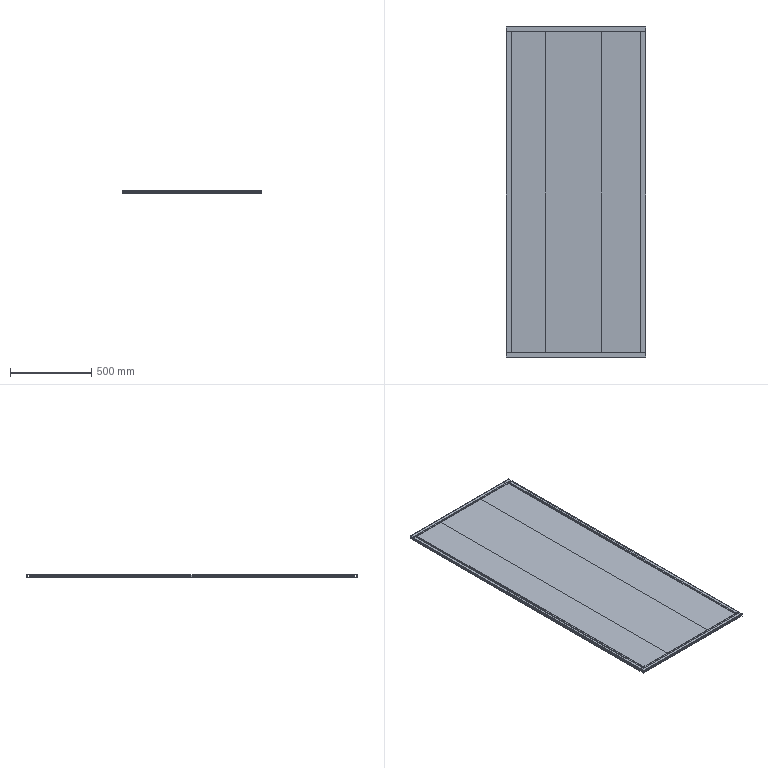Part | 5 solids | 175 faces | box 860 x 2036 x 18 mm | volume 17379775 mm3 | plane 106 | cylinder 69 | commonest cylinder face diameters 1.1 x24 3.6 x20 5.8 x20 1 x5